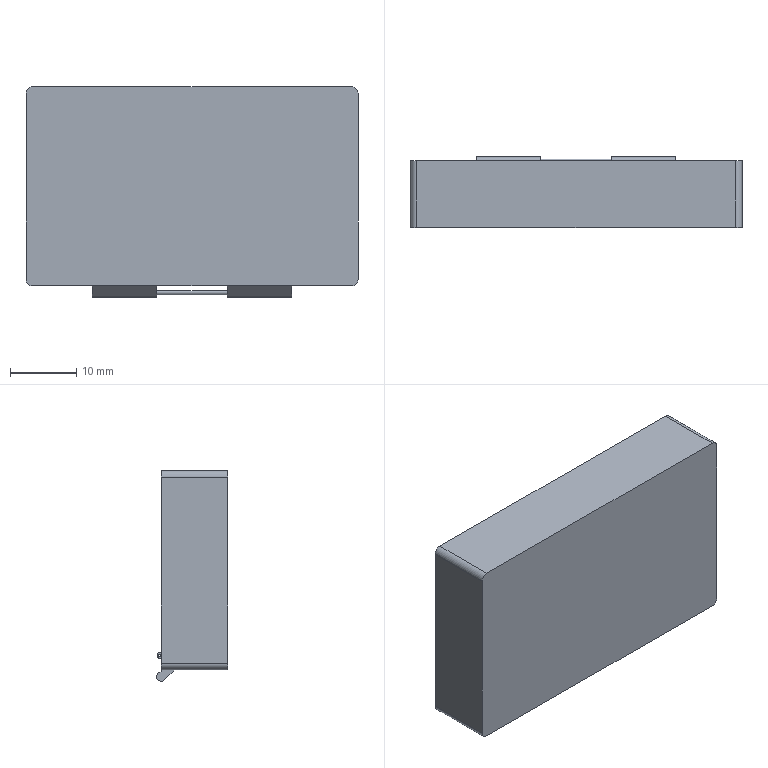Part | SolidWorks | features ICE 17, Stock 4, CirPattern 3, MoveCopyBody 3, Extrusion 1, Fillet 1, Shell 1 | 1 solid | 159 faces | box 50 x 10.7 x 31.711 mm | volume 5162 mm3 | plane 105 | cylinder 54 | commonest cylinder face diameters 6.2 x15 6 x13 5.996 x6 6.166 x6 0.4 x4 2 x4